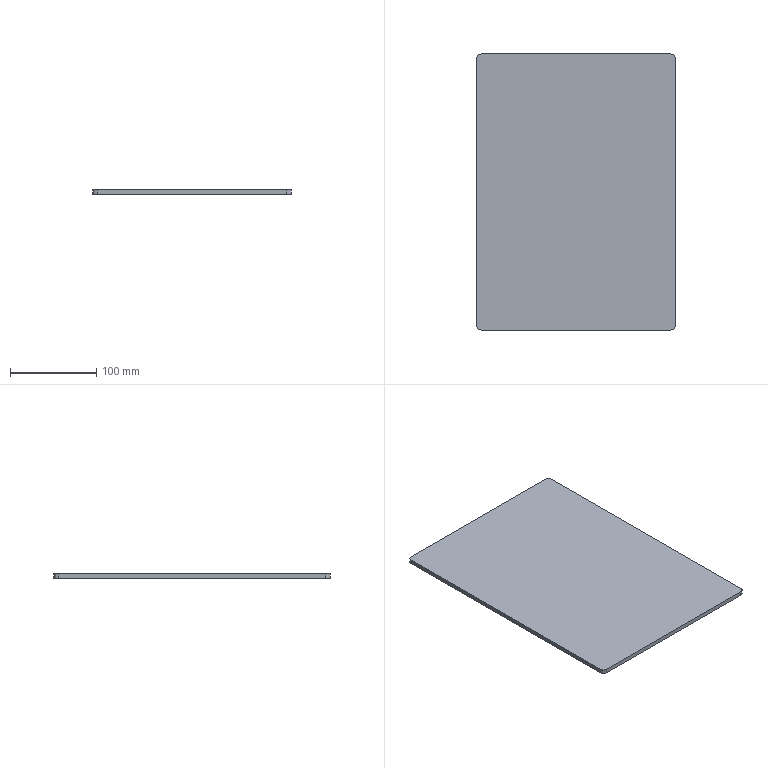Part | STEP file | 001-002-Face Plate-5 | 1 solid | 10 faces | box 230 x 320 x 5 mm | volume 367893 mm3 | plane 6 | cylinder 4 | commonest cylinder face diameters 10 x4
STEP:
#1=CARTESIAN_POINT('',(0.,0.,0.));
#2=DIRECTION('',(0.,0.,1.));
#3=DIRECTION('',(1.,0.,0.));
#4=AXIS2_PLACEMENT_3D('',#1,#2,#3);
#5=CARTESIAN_POINT('',(115.,-155.,0.));
#6=VERTEX_POINT('',#5);
#7=CARTESIAN_POINT('',(115.,155.,0.));
#8=VERTEX_POINT('',#7);
#9=CARTESIAN_POINT('',(115.,-160.,0.));
#10=DIRECTION('',(0.,1.,0.));
#11=VECTOR('',#10,1.);
#12=LINE('',#9,#11);
#13=CARTESIAN_POINT('',(115.,-160.,5.));
#14=DIRECTION('',(-1.,0.,0.));
#15=DIRECTION('',(0.,0.,1.));
#16=AXIS2_PLACEMENT_3D('',#13,#14,#15);
#17=PLANE('',#16);
#18=CARTESIAN_POINT('',(-5.,0.));
#19=DIRECTION('',(0.,1.));
#20=VECTOR('',#19,1.);
#21=LINE('',#18,#20);
#22=(GEOMETRIC_REPRESENTATION_CONTEXT(2)PARAMETRIC_REPRESENTATION_CONTEXT()REPRESENTATION_CONTEXT('',''));
#23=DEFINITIONAL_REPRESENTATION('',(#21),#22);
#24=PCURVE('',#17,#23);
#25=CARTESIAN_POINT('',(0.,0.,0.));
#26=DIRECTION('',(0.,0.,-1.));
#27=DIRECTION('',(-1.,0.,0.));
#28=AXIS2_PLACEMENT_3D('',#25,#26,#27);
#29=PLANE('',#28);
#30=CARTESIAN_POINT('',(-115.,-160.));
#31=DIRECTION('',(0.,1.));
#32=VECTOR('',#31,1.);
#33=LINE('',#30,#32);
#34=(GEOMETRIC_REPRESENTATION_CONTEXT(2)PARAMETRIC_REPRESENTATION_CONTEXT()REPRESENTATION_CONTEXT('',''));
#35=DEFINITIONAL_REPRESENTATION('',(#33),#34);
#36=PCURVE('',#29,#35);
#37=SURFACE_CURVE('',#12,(#24,#36),.PCURVE_S1.);
#38=EDGE_CURVE('',#6,#8,#37,.T.);
#39=ORIENTED_EDGE('',*,*,#38,.T.);
#40=CARTESIAN_POINT('',(115.,155.,5.));
#41=VERTEX_POINT('',#40);
#42=CARTESIAN_POINT('',(115.,155.,5.));
#43=DIRECTION('',(0.,0.,1.));
#44=VECTOR('',#43,1.);
#45=LINE('',#42,#44);
#46=CARTESIAN_POINT('',(0.,315.));
#47=DIRECTION('',(1.,0.));
#48=VECTOR('',#47,1.);
#49=LINE('',#46,#48);
#50=(GEOMETRIC_REPRESENTATION_CONTEXT(2)PARAMETRIC_REPRESENTATION_CONTEXT()REPRESENTATION_CONTEXT('',''));
#51=DEFINITIONAL_REPRESENTATION('',(#49),#50);
#52=PCURVE('',#17,#51);
#53=CARTESIAN_POINT('',(110.,155.,5.));
#54=DIRECTION('',(0.,0.,-1.));
#55=DIRECTION('',(-1.,0.,0.));
#56=AXIS2_PLACEMENT_3D('',#53,#54,#55);
#57=CYLINDRICAL_SURFACE('',#56,5.);
#58=CARTESIAN_POINT('',(3.142,0.));
#59=DIRECTION('',(0.,-1.));
#60=VECTOR('',#59,1.);
#61=LINE('',#58,#60);
#62=(GEOMETRIC_REPRESENTATION_CONTEXT(2)PARAMETRIC_REPRESENTATION_CONTEXT()REPRESENTATION_CONTEXT('',''));
#63=DEFINITIONAL_REPRESENTATION('',(#61),#62);
#64=PCURVE('',#57,#63);
#65=SURFACE_CURVE('',#45,(#52,#64),.PCURVE_S1.);
#66=EDGE_CURVE('',#8,#41,#65,.T.);
#67=ORIENTED_EDGE('',*,*,#66,.T.);
#68=CARTESIAN_POINT('',(115.,-155.,5.));
#69=VERTEX_POINT('',#68);
#70=CARTESIAN_POINT('',(115.,-160.,5.));
#71=DIRECTION('',(0.,1.,0.));
#72=VECTOR('',#71,1.);
#73=LINE('',#70,#72);
#74=CARTESIAN_POINT('',(0.,0.));
#75=DIRECTION('',(0.,1.));
#76=VECTOR('',#75,1.);
#77=LINE('',#74,#76);
#78=(GEOMETRIC_REPRESENTATION_CONTEXT(2)PARAMETRIC_REPRESENTATION_CONTEXT()REPRESENTATION_CONTEXT('',''));
#79=DEFINITIONAL_REPRESENTATION('',(#77),#78);
#80=PCURVE('',#17,#79);
#81=CARTESIAN_POINT('',(0.,0.,5.));
#82=DIRECTION('',(0.,0.,-1.));
#83=DIRECTION('',(-1.,0.,0.));
#84=AXIS2_PLACEMENT_3D('',#81,#82,#83);
#85=PLANE('',#84);
#86=CARTESIAN_POINT('',(-115.,-160.));
#87=DIRECTION('',(0.,1.));
#88=VECTOR('',#87,1.);
#89=LINE('',#86,#88);
#90=(GEOMETRIC_REPRESENTATION_CONTEXT(2)PARAMETRIC_REPRESENTATION_CONTEXT()REPRESENTATION_CONTEXT('',''));
#91=DEFINITIONAL_REPRESENTATION('',(#89),#90);
#92=PCURVE('',#85,#91);
#93=SURFACE_CURVE('',#73,(#80,#92),.PCURVE_S1.);
#94=EDGE_CURVE('',#69,#41,#93,.T.);
#95=ORIENTED_EDGE('',*,*,#94,.F.);
#96=CARTESIAN_POINT('',(115.,-155.,5.));
#97=DIRECTION('',(0.,0.,-1.));
#98=VECTOR('',#97,1.);
#99=LINE('',#96,#98);
#100=CARTESIAN_POINT('',(0.,5.));
#101=DIRECTION('',(-1.,0.));
#102=VECTOR('',#101,1.);
#103=LINE('',#100,#102);
#104=(GEOMETRIC_REPRESENTATION_CONTEXT(2)PARAMETRIC_REPRESENTATION_CONTEXT()REPRESENTATION_CONTEXT('',''));
#105=DEFINITIONAL_REPRESENTATION('',(#103),#104);
#106=PCURVE('',#17,#105);
#107=CARTESIAN_POINT('',(110.,-155.,5.));
#108=DIRECTION('',(0.,0.,-1.));
#109=DIRECTION('',(-1.,0.,0.));
#110=AXIS2_PLACEMENT_3D('',#107,#108,#109);
#111=CYLINDRICAL_SURFACE('',#110,5.);
#112=CARTESIAN_POINT('',(3.142,0.));
#113=DIRECTION('',(0.,1.));
#114=VECTOR('',#113,1.);
#115=LINE('',#112,#114);
#116=(GEOMETRIC_REPRESENTATION_CONTEXT(2)PARAMETRIC_REPRESENTATION_CONTEXT()REPRESENTATION_CONTEXT('',''));
#117=DEFINITIONAL_REPRESENTATION('',(#115),#116);
#118=PCURVE('',#111,#117);
#119=SURFACE_CURVE('',#99,(#106,#118),.PCURVE_S1.);
#120=EDGE_CURVE('',#69,#6,#119,.T.);
#121=ORIENTED_EDGE('',*,*,#120,.T.);
#122=EDGE_LOOP('',(#39,#67,#95,#121));
#123=FACE_BOUND('',#122,.T.);
#124=ADVANCED_FACE('',(#123),#17,.F.);
#125=CARTESIAN_POINT('',(110.,160.,0.));
#126=VERTEX_POINT('',#125);
#127=CARTESIAN_POINT('',(-110.,160.,0.));
#128=VERTEX_POINT('',#127);
#129=CARTESIAN_POINT('',(-115.,160.,0.));
#130=DIRECTION('',(-1.,0.,0.));
#131=VECTOR('',#130,1.);
#132=LINE('',#129,#131);
#133=CARTESIAN_POINT('',(-115.,160.,5.));
#134=DIRECTION('',(0.,-1.,0.));
#135=DIRECTION('',(0.,0.,-1.));
#136=AXIS2_PLACEMENT_3D('',#133,#134,#135);
#137=PLANE('',#136);
#138=CARTESIAN_POINT('',(5.,0.));
#139=DIRECTION('',(0.,-1.));
#140=VECTOR('',#139,1.);
#141=LINE('',#138,#140);
#142=(GEOMETRIC_REPRESENTATION_CONTEXT(2)PARAMETRIC_REPRESENTATION_CONTEXT()REPRESENTATION_CONTEXT('',''));
#143=DEFINITIONAL_REPRESENTATION('',(#141),#142);
#144=PCURVE('',#137,#143);
#145=CARTESIAN_POINT('',(115.,160.));
#146=DIRECTION('',(1.,0.));
#147=VECTOR('',#146,1.);
#148=LINE('',#145,#147);
#149=(GEOMETRIC_REPRESENTATION_CONTEXT(2)PARAMETRIC_REPRESENTATION_CONTEXT()REPRESENTATION_CONTEXT('',''));
#150=DEFINITIONAL_REPRESENTATION('',(#148),#149);
#151=PCURVE('',#29,#150);
#152=SURFACE_CURVE('',#132,(#144,#151),.PCURVE_S1.);
#153=EDGE_CURVE('',#126,#128,#152,.T.);
#154=ORIENTED_EDGE('',*,*,#153,.T.);
#155=CARTESIAN_POINT('',(-110.,160.,5.));
#156=VERTEX_POINT('',#155);
#157=CARTESIAN_POINT('',(-110.,160.,5.));
#158=DIRECTION('',(0.,0.,1.));
#159=VECTOR('',#158,1.);
#160=LINE('',#157,#159);
#161=CARTESIAN_POINT('',(0.,5.));
#162=DIRECTION('',(-1.,0.));
#163=VECTOR('',#162,1.);
#164=LINE('',#161,#163);
#165=(GEOMETRIC_REPRESENTATION_CONTEXT(2)PARAMETRIC_REPRESENTATION_CONTEXT()REPRESENTATION_CONTEXT('',''));
#166=DEFINITIONAL_REPRESENTATION('',(#164),#165);
#167=PCURVE('',#137,#166);
#168=CARTESIAN_POINT('',(-110.,155.,5.));
#169=DIRECTION('',(0.,0.,-1.));
#170=DIRECTION('',(-1.,0.,0.));
#171=AXIS2_PLACEMENT_3D('',#168,#169,#170);
#172=CYLINDRICAL_SURFACE('',#171,5.);
#173=CARTESIAN_POINT('',(1.571,0.));
#174=DIRECTION('',(0.,-1.));
#175=VECTOR('',#174,1.);
#176=LINE('',#173,#175);
#177=(GEOMETRIC_REPRESENTATION_CONTEXT(2)PARAMETRIC_REPRESENTATION_CONTEXT()REPRESENTATION_CONTEXT('',''));
#178=DEFINITIONAL_REPRESENTATION('',(#176),#177);
#179=PCURVE('',#172,#178);
#180=SURFACE_CURVE('',#160,(#167,#179),.PCURVE_S1.);
#181=EDGE_CURVE('',#128,#156,#180,.T.);
#182=ORIENTED_EDGE('',*,*,#181,.T.);
#183=CARTESIAN_POINT('',(110.,160.,5.));
#184=VERTEX_POINT('',#183);
#185=CARTESIAN_POINT('',(-115.,160.,5.));
#186=DIRECTION('',(-1.,0.,0.));
#187=VECTOR('',#186,1.);
#188=LINE('',#185,#187);
#189=CARTESIAN_POINT('',(0.,0.));
#190=DIRECTION('',(0.,-1.));
#191=VECTOR('',#190,1.);
#192=LINE('',#189,#191);
#193=(GEOMETRIC_REPRESENTATION_CONTEXT(2)PARAMETRIC_REPRESENTATION_CONTEXT()REPRESENTATION_CONTEXT('',''));
#194=DEFINITIONAL_REPRESENTATION('',(#192),#193);
#195=PCURVE('',#137,#194);
#196=CARTESIAN_POINT('',(115.,160.));
#197=DIRECTION('',(1.,0.));
#198=VECTOR('',#197,1.);
#199=LINE('',#196,#198);
#200=(GEOMETRIC_REPRESENTATION_CONTEXT(2)PARAMETRIC_REPRESENTATION_CONTEXT()REPRESENTATION_CONTEXT('',''));
#201=DEFINITIONAL_REPRESENTATION('',(#199),#200);
#202=PCURVE('',#85,#201);
#203=SURFACE_CURVE('',#188,(#195,#202),.PCURVE_S1.);
#204=EDGE_CURVE('',#184,#156,#203,.T.);
#205=ORIENTED_EDGE('',*,*,#204,.F.);
#206=CARTESIAN_POINT('',(110.,160.,5.));
#207=DIRECTION('',(0.,0.,-1.));
#208=VECTOR('',#207,1.);
#209=LINE('',#206,#208);
#210=CARTESIAN_POINT('',(0.,225.));
#211=DIRECTION('',(1.,0.));
#212=VECTOR('',#211,1.);
#213=LINE('',#210,#212);
#214=(GEOMETRIC_REPRESENTATION_CONTEXT(2)PARAMETRIC_REPRESENTATION_CONTEXT()REPRESENTATION_CONTEXT('',''));
#215=DEFINITIONAL_REPRESENTATION('',(#213),#214);
#216=PCURVE('',#137,#215);
#217=CARTESIAN_POINT('',(1.571,0.));
#218=DIRECTION('',(0.,1.));
#219=VECTOR('',#218,1.);
#220=LINE('',#217,#219);
#221=(GEOMETRIC_REPRESENTATION_CONTEXT(2)PARAMETRIC_REPRESENTATION_CONTEXT()REPRESENTATION_CONTEXT('',''));
#222=DEFINITIONAL_REPRESENTATION('',(#220),#221);
#223=PCURVE('',#57,#222);
#224=SURFACE_CURVE('',#209,(#216,#223),.PCURVE_S1.);
#225=EDGE_CURVE('',#184,#126,#224,.T.);
#226=ORIENTED_EDGE('',*,*,#225,.T.);
#227=EDGE_LOOP('',(#154,#182,#205,#226));
#228=FACE_BOUND('',#227,.T.);
#229=ADVANCED_FACE('',(#228),#137,.F.);
#230=CARTESIAN_POINT('',(-115.,155.,0.));
#231=VERTEX_POINT('',#230);
#232=CARTESIAN_POINT('',(-115.,-155.,0.));
#233=VERTEX_POINT('',#232);
#234=CARTESIAN_POINT('',(-115.,-160.,0.));
#235=DIRECTION('',(0.,-1.,0.));
#236=VECTOR('',#235,1.);
#237=LINE('',#234,#236);
#238=CARTESIAN_POINT('',(-115.,-160.,5.));
#239=DIRECTION('',(1.,0.,0.));
#240=DIRECTION('',(0.,0.,-1.));
#241=AXIS2_PLACEMENT_3D('',#238,#239,#240);
#242=PLANE('',#241);
#243=CARTESIAN_POINT('',(5.,0.));
#244=DIRECTION('',(0.,-1.));
#245=VECTOR('',#244,1.);
#246=LINE('',#243,#245);
#247=(GEOMETRIC_REPRESENTATION_CONTEXT(2)PARAMETRIC_REPRESENTATION_CONTEXT()REPRESENTATION_CONTEXT('',''));
#248=DEFINITIONAL_REPRESENTATION('',(#246),#247);
#249=PCURVE('',#242,#248);
#250=CARTESIAN_POINT('',(115.,-160.));
#251=DIRECTION('',(0.,-1.));
#252=VECTOR('',#251,1.);
#253=LINE('',#250,#252);
#254=(GEOMETRIC_REPRESENTATION_CONTEXT(2)PARAMETRIC_REPRESENTATION_CONTEXT()REPRESENTATION_CONTEXT('',''));
#255=DEFINITIONAL_REPRESENTATION('',(#253),#254);
#256=PCURVE('',#29,#255);
#257=SURFACE_CURVE('',#237,(#249,#256),.PCURVE_S1.);
#258=EDGE_CURVE('',#231,#233,#257,.T.);
#259=ORIENTED_EDGE('',*,*,#258,.T.);
#260=CARTESIAN_POINT('',(-115.,-155.,5.));
#261=VERTEX_POINT('',#260);
#262=CARTESIAN_POINT('',(-115.,-155.,5.));
#263=DIRECTION('',(0.,0.,1.));
#264=VECTOR('',#263,1.);
#265=LINE('',#262,#264);
#266=CARTESIAN_POINT('',(0.,5.));
#267=DIRECTION('',(-1.,0.));
#268=VECTOR('',#267,1.);
#269=LINE('',#266,#268);
#270=(GEOMETRIC_REPRESENTATION_CONTEXT(2)PARAMETRIC_REPRESENTATION_CONTEXT()REPRESENTATION_CONTEXT('',''));
#271=DEFINITIONAL_REPRESENTATION('',(#269),#270);
#272=PCURVE('',#242,#271);
#273=CARTESIAN_POINT('',(-110.,-155.,5.));
#274=DIRECTION('',(0.,0.,-1.));
#275=DIRECTION('',(-1.,0.,0.));
#276=AXIS2_PLACEMENT_3D('',#273,#274,#275);
#277=CYLINDRICAL_SURFACE('',#276,5.);
#278=CARTESIAN_POINT('',(6.283,0.));
#279=DIRECTION('',(0.,-1.));
#280=VECTOR('',#279,1.);
#281=LINE('',#278,#280);
#282=(GEOMETRIC_REPRESENTATION_CONTEXT(2)PARAMETRIC_REPRESENTATION_CONTEXT()REPRESENTATION_CONTEXT('',''));
#283=DEFINITIONAL_REPRESENTATION('',(#281),#282);
#284=PCURVE('',#277,#283);
#285=SURFACE_CURVE('',#265,(#272,#284),.PCURVE_S1.);
#286=EDGE_CURVE('',#233,#261,#285,.T.);
#287=ORIENTED_EDGE('',*,*,#286,.T.);
#288=CARTESIAN_POINT('',(-115.,155.,5.));
#289=VERTEX_POINT('',#288);
#290=CARTESIAN_POINT('',(-115.,-160.,5.));
#291=DIRECTION('',(0.,-1.,0.));
#292=VECTOR('',#291,1.);
#293=LINE('',#290,#292);
#294=CARTESIAN_POINT('',(0.,0.));
#295=DIRECTION('',(0.,-1.));
#296=VECTOR('',#295,1.);
#297=LINE('',#294,#296);
#298=(GEOMETRIC_REPRESENTATION_CONTEXT(2)PARAMETRIC_REPRESENTATION_CONTEXT()REPRESENTATION_CONTEXT('',''));
#299=DEFINITIONAL_REPRESENTATION('',(#297),#298);
#300=PCURVE('',#242,#299);
#301=CARTESIAN_POINT('',(115.,-160.));
#302=DIRECTION('',(0.,-1.));
#303=VECTOR('',#302,1.);
#304=LINE('',#301,#303);
#305=(GEOMETRIC_REPRESENTATION_CONTEXT(2)PARAMETRIC_REPRESENTATION_CONTEXT()REPRESENTATION_CONTEXT('',''));
#306=DEFINITIONAL_REPRESENTATION('',(#304),#305);
#307=PCURVE('',#85,#306);
#308=SURFACE_CURVE('',#293,(#300,#307),.PCURVE_S1.);
#309=EDGE_CURVE('',#289,#261,#308,.T.);
#310=ORIENTED_EDGE('',*,*,#309,.F.);
#311=CARTESIAN_POINT('',(-115.,155.,5.));
#312=DIRECTION('',(0.,0.,-1.));
#313=VECTOR('',#312,1.);
#314=LINE('',#311,#313);
#315=CARTESIAN_POINT('',(0.,315.));
#316=DIRECTION('',(1.,0.));
#317=VECTOR('',#316,1.);
#318=LINE('',#315,#317);
#319=(GEOMETRIC_REPRESENTATION_CONTEXT(2)PARAMETRIC_REPRESENTATION_CONTEXT()REPRESENTATION_CONTEXT('',''));
#320=DEFINITIONAL_REPRESENTATION('',(#318),#319);
#321=PCURVE('',#242,#320);
#322=CARTESIAN_POINT('',(0.,0.));
#323=DIRECTION('',(0.,1.));
#324=VECTOR('',#323,1.);
#325=LINE('',#322,#324);
#326=(GEOMETRIC_REPRESENTATION_CONTEXT(2)PARAMETRIC_REPRESENTATION_CONTEXT()REPRESENTATION_CONTEXT('',''));
#327=DEFINITIONAL_REPRESENTATION('',(#325),#326);
#328=PCURVE('',#172,#327);
#329=SURFACE_CURVE('',#314,(#321,#328),.PCURVE_S1.);
#330=EDGE_CURVE('',#289,#231,#329,.T.);
#331=ORIENTED_EDGE('',*,*,#330,.T.);
#332=EDGE_LOOP('',(#259,#287,#310,#331));
#333=FACE_BOUND('',#332,.T.);
#334=ADVANCED_FACE('',(#333),#242,.F.);
#335=CARTESIAN_POINT('',(-110.,-160.,5.));
#336=VERTEX_POINT('',#335);
#337=CARTESIAN_POINT('',(110.,-160.,5.));
#338=VERTEX_POINT('',#337);
#339=CARTESIAN_POINT('',(-115.,-160.,5.));
#340=DIRECTION('',(1.,0.,0.));
#341=VECTOR('',#340,1.);
#342=LINE('',#339,#341);
#343=CARTESIAN_POINT('',(-115.,-160.,5.));
#344=DIRECTION('',(0.,1.,0.));
#345=DIRECTION('',(0.,0.,1.));
#346=AXIS2_PLACEMENT_3D('',#343,#344,#345);
#347=PLANE('',#346);
#348=CARTESIAN_POINT('',(0.,0.));
#349=DIRECTION('',(0.,1.));
#350=VECTOR('',#349,1.);
#351=LINE('',#348,#350);
#352=(GEOMETRIC_REPRESENTATION_CONTEXT(2)PARAMETRIC_REPRESENTATION_CONTEXT()REPRESENTATION_CONTEXT('',''));
#353=DEFINITIONAL_REPRESENTATION('',(#351),#352);
#354=PCURVE('',#347,#353);
#355=CARTESIAN_POINT('',(115.,-160.));
#356=DIRECTION('',(-1.,0.));
#357=VECTOR('',#356,1.);
#358=LINE('',#355,#357);
#359=(GEOMETRIC_REPRESENTATION_CONTEXT(2)PARAMETRIC_REPRESENTATION_CONTEXT()REPRESENTATION_CONTEXT('',''));
#360=DEFINITIONAL_REPRESENTATION('',(#358),#359);
#361=PCURVE('',#85,#360);
#362=SURFACE_CURVE('',#342,(#354,#361),.PCURVE_S1.);
#363=EDGE_CURVE('',#336,#338,#362,.T.);
#364=ORIENTED_EDGE('',*,*,#363,.F.);
#365=CARTESIAN_POINT('',(-110.,-160.,0.));
#366=VERTEX_POINT('',#365);
#367=CARTESIAN_POINT('',(-110.,-160.,5.));
#368=DIRECTION('',(0.,0.,-1.));
#369=VECTOR('',#368,1.);
#370=LINE('',#367,#369);
#371=CARTESIAN_POINT('',(0.,5.));
#372=DIRECTION('',(-1.,0.));
#373=VECTOR('',#372,1.);
#374=LINE('',#371,#373);
#375=(GEOMETRIC_REPRESENTATION_CONTEXT(2)PARAMETRIC_REPRESENTATION_CONTEXT()REPRESENTATION_CONTEXT('',''));
#376=DEFINITIONAL_REPRESENTATION('',(#374),#375);
#377=PCURVE('',#347,#376);
#378=CARTESIAN_POINT('',(4.712,0.));
#379=DIRECTION('',(0.,1.));
#380=VECTOR('',#379,1.);
#381=LINE('',#378,#380);
#382=(GEOMETRIC_REPRESENTATION_CONTEXT(2)PARAMETRIC_REPRESENTATION_CONTEXT()REPRESENTATION_CONTEXT('',''));
#383=DEFINITIONAL_REPRESENTATION('',(#381),#382);
#384=PCURVE('',#277,#383);
#385=SURFACE_CURVE('',#370,(#377,#384),.PCURVE_S1.);
#386=EDGE_CURVE('',#336,#366,#385,.T.);
#387=ORIENTED_EDGE('',*,*,#386,.T.);
#388=CARTESIAN_POINT('',(110.,-160.,0.));
#389=VERTEX_POINT('',#388);
#390=CARTESIAN_POINT('',(-115.,-160.,0.));
#391=DIRECTION('',(1.,0.,0.));
#392=VECTOR('',#391,1.);
#393=LINE('',#390,#392);
#394=CARTESIAN_POINT('',(-5.,0.));
#395=DIRECTION('',(0.,1.));
#396=VECTOR('',#395,1.);
#397=LINE('',#394,#396);
#398=(GEOMETRIC_REPRESENTATION_CONTEXT(2)PARAMETRIC_REPRESENTATION_CONTEXT()REPRESENTATION_CONTEXT('',''));
#399=DEFINITIONAL_REPRESENTATION('',(#397),#398);
#400=PCURVE('',#347,#399);
#401=CARTESIAN_POINT('',(115.,-160.));
#402=DIRECTION('',(-1.,0.));
#403=VECTOR('',#402,1.);
#404=LINE('',#401,#403);
#405=(GEOMETRIC_REPRESENTATION_CONTEXT(2)PARAMETRIC_REPRESENTATION_CONTEXT()REPRESENTATION_CONTEXT('',''));
#406=DEFINITIONAL_REPRESENTATION('',(#404),#405);
#407=PCURVE('',#29,#406);
#408=SURFACE_CURVE('',#393,(#400,#407),.PCURVE_S1.);
#409=EDGE_CURVE('',#366,#389,#408,.T.);
#410=ORIENTED_EDGE('',*,*,#409,.T.);
#411=CARTESIAN_POINT('',(110.,-160.,5.));
#412=DIRECTION('',(0.,0.,1.));
#413=VECTOR('',#412,1.);
#414=LINE('',#411,#413);
#415=CARTESIAN_POINT('',(0.,225.));
#416=DIRECTION('',(1.,0.));
#417=VECTOR('',#416,1.);
#418=LINE('',#415,#417);
#419=(GEOMETRIC_REPRESENTATION_CONTEXT(2)PARAMETRIC_REPRESENTATION_CONTEXT()REPRESENTATION_CONTEXT('',''));
#420=DEFINITIONAL_REPRESENTATION('',(#418),#419);
#421=PCURVE('',#347,#420);
#422=CARTESIAN_POINT('',(4.712,0.));
#423=DIRECTION('',(0.,-1.));
#424=VECTOR('',#423,1.);
#425=LINE('',#422,#424);
#426=(GEOMETRIC_REPRESENTATION_CONTEXT(2)PARAMETRIC_REPRESENTATION_CONTEXT()REPRESENTATION_CONTEXT('',''));
#427=DEFINITIONAL_REPRESENTATION('',(#425),#426);
#428=PCURVE('',#111,#427);
#429=SURFACE_CURVE('',#414,(#421,#428),.PCURVE_S1.);
#430=EDGE_CURVE('',#389,#338,#429,.T.);
#431=ORIENTED_EDGE('',*,*,#430,.T.);
#432=EDGE_LOOP('',(#364,#387,#410,#431));
#433=FACE_BOUND('',#432,.T.);
#434=ADVANCED_FACE('',(#433),#347,.F.);
#435=ORIENTED_EDGE('',*,*,#309,.T.);
#436=CARTESIAN_POINT('',(-110.,-155.,5.));
#437=DIRECTION('',(0.,0.,1.));
#438=DIRECTION('',(-1.,0.,0.));
#439=AXIS2_PLACEMENT_3D('',#436,#437,#438);
#440=CIRCLE('',#439,5.);
#441=CARTESIAN_POINT('',(115.,-155.));
#442=CARTESIAN_POINT('',(115.,-163.66));
#443=CARTESIAN_POINT('',(107.5,-159.33));
#444=CARTESIAN_POINT('',(100.,-155.));
#445=CARTESIAN_POINT('',(107.5,-150.67));
#446=CARTESIAN_POINT('',(115.,-146.34));
#447=CARTESIAN_POINT('',(115.,-155.));
#448=(BOUNDED_CURVE()B_SPLINE_CURVE(2,(#441,#442,#443,#444,#445,#446,#447),.UNSPECIFIED.,.T.,.F.)B_SPLINE_CURVE_WITH_KNOTS((1,2,2,2,2,1),(-2.094,0.,2.094,4.189,6.283,8.378),.UNSPECIFIED.)CURVE()GEOMETRIC_REPRESENTATION_ITEM()RATIONAL_B_SPLINE_CURVE((1.,0.5,1.,0.5,1.,0.5,1.))REPRESENTATION_ITEM(''));
#449=(GEOMETRIC_REPRESENTATION_CONTEXT(2)PARAMETRIC_REPRESENTATION_CONTEXT()REPRESENTATION_CONTEXT('',''));
#450=DEFINITIONAL_REPRESENTATION('',(#448),#449);
#451=PCURVE('',#85,#450);
#452=CARTESIAN_POINT('',(6.283,0.));
#453=DIRECTION('',(-1.,0.));
#454=VECTOR('',#453,1.);
#455=LINE('',#452,#454);
#456=(GEOMETRIC_REPRESENTATION_CONTEXT(2)PARAMETRIC_REPRESENTATION_CONTEXT()REPRESENTATION_CONTEXT('',''));
#457=DEFINITIONAL_REPRESENTATION('',(#455),#456);
#458=PCURVE('',#277,#457);
#459=SURFACE_CURVE('',#440,(#451,#458),.PCURVE_S1.);
#460=EDGE_CURVE('',#261,#336,#459,.T.);
#461=ORIENTED_EDGE('',*,*,#460,.T.);
#462=ORIENTED_EDGE('',*,*,#363,.T.);
#463=CARTESIAN_POINT('',(110.,-155.,5.));
#464=DIRECTION('',(0.,0.,1.));
#465=DIRECTION('',(-1.,0.,0.));
#466=AXIS2_PLACEMENT_3D('',#463,#464,#465);
#467=CIRCLE('',#466,5.);
#468=CARTESIAN_POINT('',(-105.,-155.));
#469=CARTESIAN_POINT('',(-105.,-163.66));
#470=CARTESIAN_POINT('',(-112.5,-159.33));
#471=CARTESIAN_POINT('',(-120.,-155.));
#472=CARTESIAN_POINT('',(-112.5,-150.67));
#473=CARTESIAN_POINT('',(-105.,-146.34));
#474=CARTESIAN_POINT('',(-105.,-155.));
#475=(BOUNDED_CURVE()B_SPLINE_CURVE(2,(#468,#469,#470,#471,#472,#473,#474),.UNSPECIFIED.,.T.,.F.)B_SPLINE_CURVE_WITH_KNOTS((1,2,2,2,2,1),(-2.094,0.,2.094,4.189,6.283,8.378),.UNSPECIFIED.)CURVE()GEOMETRIC_REPRESENTATION_ITEM()RATIONAL_B_SPLINE_CURVE((1.,0.5,1.,0.5,1.,0.5,1.))REPRESENTATION_ITEM(''));
#476=(GEOMETRIC_REPRESENTATION_CONTEXT(2)PARAMETRIC_REPRESENTATION_CONTEXT()REPRESENTATION_CONTEXT('',''));
#477=DEFINITIONAL_REPRESENTATION('',(#475),#476);
#478=PCURVE('',#85,#477);
#479=CARTESIAN_POINT('',(6.283,0.));
#480=DIRECTION('',(-1.,0.));
#481=VECTOR('',#480,1.);
#482=LINE('',#479,#481);
#483=(GEOMETRIC_REPRESENTATION_CONTEXT(2)PARAMETRIC_REPRESENTATION_CONTEXT()REPRESENTATION_CONTEXT('',''));
#484=DEFINITIONAL_REPRESENTATION('',(#482),#483);
#485=PCURVE('',#111,#484);
#486=SURFACE_CURVE('',#467,(#478,#485),.PCURVE_S1.);
#487=EDGE_CURVE('',#338,#69,#486,.T.);
#488=ORIENTED_EDGE('',*,*,#487,.T.);
#489=ORIENTED_EDGE('',*,*,#94,.T.);
#490=CARTESIAN_POINT('',(110.,155.,5.));
#491=DIRECTION('',(0.,0.,1.));
#492=DIRECTION('',(-1.,0.,0.));
#493=AXIS2_PLACEMENT_3D('',#490,#491,#492);
#494=CIRCLE('',#493,5.);
#495=CARTESIAN_POINT('',(-105.,155.));
#496=CARTESIAN_POINT('',(-105.,146.34));
#497=CARTESIAN_POINT('',(-112.5,150.67));
#498=CARTESIAN_POINT('',(-120.,155.));
#499=CARTESIAN_POINT('',(-112.5,159.33));
#500=CARTESIAN_POINT('',(-105.,163.66));
#501=CARTESIAN_POINT('',(-105.,155.));
#502=(BOUNDED_CURVE()B_SPLINE_CURVE(2,(#495,#496,#497,#498,#499,#500,#501),.UNSPECIFIED.,.T.,.F.)B_SPLINE_CURVE_WITH_KNOTS((1,2,2,2,2,1),(-2.094,0.,2.094,4.189,6.283,8.378),.UNSPECIFIED.)CURVE()GEOMETRIC_REPRESENTATION_ITEM()RATIONAL_B_SPLINE_CURVE((1.,0.5,1.,0.5,1.,0.5,1.))REPRESENTATION_ITEM(''));
#503=(GEOMETRIC_REPRESENTATION_CONTEXT(2)PARAMETRIC_REPRESENTATION_CONTEXT()REPRESENTATION_CONTEXT('',''));
#504=DEFINITIONAL_REPRESENTATION('',(#502),#503);
#505=PCURVE('',#85,#504);
#506=CARTESIAN_POINT('',(6.283,0.));
#507=DIRECTION('',(-1.,0.));
#508=VECTOR('',#507,1.);
#509=LINE('',#506,#508);
#510=(GEOMETRIC_REPRESENTATION_CONTEXT(2)PARAMETRIC_REPRESENTATION_CONTEXT()REPRESENTATION_CONTEXT('',''));
#511=DEFINITIONAL_REPRESENTATION('',(#509),#510);
#512=PCURVE('',#57,#511);
#513=SURFACE_CURVE('',#494,(#505,#512),.PCURVE_S1.);
#514=EDGE_CURVE('',#41,#184,#513,.T.);
#515=ORIENTED_EDGE('',*,*,#514,.T.);
#516=ORIENTED_EDGE('',*,*,#204,.T.);
#517=CARTESIAN_POINT('',(-110.,155.,5.));
#518=DIRECTION('',(0.,0.,1.));
#519=DIRECTION('',(-1.,0.,0.));
#520=AXIS2_PLACEMENT_3D('',#517,#518,#519);
#521=CIRCLE('',#520,5.);
#522=CARTESIAN_POINT('',(115.,155.));
#523=CARTESIAN_POINT('',(115.,146.34));
#524=CARTESIAN_POINT('',(107.5,150.67));
#525=CARTESIAN_POINT('',(100.,155.));
#526=CARTESIAN_POINT('',(107.5,159.33));
#527=CARTESIAN_POINT('',(115.,163.66));
#528=CARTESIAN_POINT('',(115.,155.));
#529=(BOUNDED_CURVE()B_SPLINE_CURVE(2,(#522,#523,#524,#525,#526,#527,#528),.UNSPECIFIED.,.T.,.F.)B_SPLINE_CURVE_WITH_KNOTS((1,2,2,2,2,1),(-2.094,0.,2.094,4.189,6.283,8.378),.UNSPECIFIED.)CURVE()GEOMETRIC_REPRESENTATION_ITEM()RATIONAL_B_SPLINE_CURVE((1.,0.5,1.,0.5,1.,0.5,1.))REPRESENTATION_ITEM(''));
#530=(GEOMETRIC_REPRESENTATION_CONTEXT(2)PARAMETRIC_REPRESENTATION_CONTEXT()REPRESENTATION_CONTEXT('',''));
#531=DEFINITIONAL_REPRESENTATION('',(#529),#530);
#532=PCURVE('',#85,#531);
#533=CARTESIAN_POINT('',(6.283,0.));
#534=DIRECTION('',(-1.,0.));
#535=VECTOR('',#534,1.);
#536=LINE('',#533,#535);
#537=(GEOMETRIC_REPRESENTATION_CONTEXT(2)PARAMETRIC_REPRESENTATION_CONTEXT()REPRESENTATION_CONTEXT('',''));
#538=DEFINITIONAL_REPRESENTATION('',(#536),#537);
#539=PCURVE('',#172,#538);
#540=SURFACE_CURVE('',#521,(#532,#539),.PCURVE_S1.);
#541=EDGE_CURVE('',#156,#289,#540,.T.);
#542=ORIENTED_EDGE('',*,*,#541,.T.);
#543=EDGE_LOOP('',(#435,#461,#462,#488,#489,#515,#516,#542));
#544=FACE_BOUND('',#543,.T.);
#545=ADVANCED_FACE('',(#544),#85,.F.);
#546=ORIENTED_EDGE('',*,*,#409,.F.);
#547=CARTESIAN_POINT('',(-110.,-155.,0.));
#548=DIRECTION('',(0.,0.,-1.));
#549=DIRECTION('',(-1.,0.,0.));
#550=AXIS2_PLACEMENT_3D('',#547,#548,#549);
#551=CIRCLE('',#550,5.);
#552=CARTESIAN_POINT('',(110.,-155.));
#553=DIRECTION('',(1.,0.));
#554=AXIS2_PLACEMENT_2D('',#552,#553);
#555=CIRCLE('',#554,5.);
#556=(GEOMETRIC_REPRESENTATION_CONTEXT(2)PARAMETRIC_REPRESENTATION_CONTEXT()REPRESENTATION_CONTEXT('',''));
#557=DEFINITIONAL_REPRESENTATION('',(#555),#556);
#558=PCURVE('',#29,#557);
#559=CARTESIAN_POINT('',(0.,5.));
#560=DIRECTION('',(1.,0.));
#561=VECTOR('',#560,1.);
#562=LINE('',#559,#561);
#563=(GEOMETRIC_REPRESENTATION_CONTEXT(2)PARAMETRIC_REPRESENTATION_CONTEXT()REPRESENTATION_CONTEXT('',''));
#564=DEFINITIONAL_REPRESENTATION('',(#562),#563);
#565=PCURVE('',#277,#564);
#566=SURFACE_CURVE('',#551,(#558,#565),.PCURVE_S1.);
#567=EDGE_CURVE('',#366,#233,#566,.T.);
#568=ORIENTED_EDGE('',*,*,#567,.T.);
#569=ORIENTED_EDGE('',*,*,#258,.F.);
#570=CARTESIAN_POINT('',(-110.,155.,0.));
#571=DIRECTION('',(0.,0.,-1.));
#572=DIRECTION('',(-1.,0.,0.));
#573=AXIS2_PLACEMENT_3D('',#570,#571,#572);
#574=CIRCLE('',#573,5.);
#575=CARTESIAN_POINT('',(110.,155.));
#576=DIRECTION('',(1.,0.));
#577=AXIS2_PLACEMENT_2D('',#575,#576);
#578=CIRCLE('',#577,5.);
#579=(GEOMETRIC_REPRESENTATION_CONTEXT(2)PARAMETRIC_REPRESENTATION_CONTEXT()REPRESENTATION_CONTEXT('',''));
#580=DEFINITIONAL_REPRESENTATION('',(#578),#579);
#581=PCURVE('',#29,#580);
#582=CARTESIAN_POINT('',(0.,5.));
#583=DIRECTION('',(1.,0.));
#584=VECTOR('',#583,1.);
#585=LINE('',#582,#584);
#586=(GEOMETRIC_REPRESENTATION_CONTEXT(2)PARAMETRIC_REPRESENTATION_CONTEXT()REPRESENTATION_CONTEXT('',''));
#587=DEFINITIONAL_REPRESENTATION('',(#585),#586);
#588=PCURVE('',#172,#587);
#589=SURFACE_CURVE('',#574,(#581,#588),.PCURVE_S1.);
#590=EDGE_CURVE('',#231,#128,#589,.T.);
#591=ORIENTED_EDGE('',*,*,#590,.T.);
#592=ORIENTED_EDGE('',*,*,#153,.F.);
#593=CARTESIAN_POINT('',(110.,155.,0.));
#594=DIRECTION('',(0.,0.,-1.));
#595=DIRECTION('',(-1.,0.,0.));
#596=AXIS2_PLACEMENT_3D('',#593,#594,#595);
#597=CIRCLE('',#596,5.);
#598=CARTESIAN_POINT('',(-110.,155.));
#599=DIRECTION('',(1.,0.));
#600=AXIS2_PLACEMENT_2D('',#598,#599);
#601=CIRCLE('',#600,5.);
#602=(GEOMETRIC_REPRESENTATION_CONTEXT(2)PARAMETRIC_REPRESENTATION_CONTEXT()REPRESENTATION_CONTEXT('',''));
#603=DEFINITIONAL_REPRESENTATION('',(#601),#602);
#604=PCURVE('',#29,#603);
#605=CARTESIAN_POINT('',(0.,5.));
#606=DIRECTION('',(1.,0.));
#607=VECTOR('',#606,1.);
#608=LINE('',#605,#607);
#609=(GEOMETRIC_REPRESENTATION_CONTEXT(2)PARAMETRIC_REPRESENTATION_CONTEXT()REPRESENTATION_CONTEXT('',''));
#610=DEFINITIONAL_REPRESENTATION('',(#608),#609);
#611=PCURVE('',#57,#610);
#612=SURFACE_CURVE('',#597,(#604,#611),.PCURVE_S1.);
#613=EDGE_CURVE('',#126,#8,#612,.T.);
#614=ORIENTED_EDGE('',*,*,#613,.T.);
#615=ORIENTED_EDGE('',*,*,#38,.F.);
#616=CARTESIAN_POINT('',(110.,-155.,0.));
#617=DIRECTION('',(0.,0.,-1.));
#618=DIRECTION('',(-1.,0.,0.));
#619=AXIS2_PLACEMENT_3D('',#616,#617,#618);
#620=CIRCLE('',#619,5.);
#621=CARTESIAN_POINT('',(-110.,-155.));
#622=DIRECTION('',(1.,0.));
#623=AXIS2_PLACEMENT_2D('',#621,#622);
#624=CIRCLE('',#623,5.);
#625=(GEOMETRIC_REPRESENTATION_CONTEXT(2)PARAMETRIC_REPRESENTATION_CONTEXT()REPRESENTATION_CONTEXT('',''));
#626=DEFINITIONAL_REPRESENTATION('',(#624),#625);
#627=PCURVE('',#29,#626);
#628=CARTESIAN_POINT('',(0.,5.));
#629=DIRECTION('',(1.,0.));
#630=VECTOR('',#629,1.);
#631=LINE('',#628,#630);
#632=(GEOMETRIC_REPRESENTATION_CONTEXT(2)PARAMETRIC_REPRESENTATION_CONTEXT()REPRESENTATION_CONTEXT('',''));
#633=DEFINITIONAL_REPRESENTATION('',(#631),#632);
#634=PCURVE('',#111,#633);
#635=SURFACE_CURVE('',#620,(#627,#634),.PCURVE_S1.);
#636=EDGE_CURVE('',#6,#389,#635,.T.);
#637=ORIENTED_EDGE('',*,*,#636,.T.);
#638=EDGE_LOOP('',(#546,#568,#569,#591,#592,#614,#615,#637));
#639=FACE_BOUND('',#638,.T.);
#640=ADVANCED_FACE('',(#639),#29,.T.);
#641=ORIENTED_EDGE('',*,*,#460,.F.);
#642=ORIENTED_EDGE('',*,*,#286,.F.);
#643=ORIENTED_EDGE('',*,*,#567,.F.);
#644=ORIENTED_EDGE('',*,*,#386,.F.);
#645=EDGE_LOOP('',(#641,#642,#643,#644));
#646=FACE_BOUND('',#645,.T.);
#647=ADVANCED_FACE('',(#646),#277,.T.);
#648=ORIENTED_EDGE('',*,*,#541,.F.);
#649=ORIENTED_EDGE('',*,*,#181,.F.);
#650=ORIENTED_EDGE('',*,*,#590,.F.);
#651=ORIENTED_EDGE('',*,*,#330,.F.);
#652=EDGE_LOOP('',(#648,#649,#650,#651));
#653=FACE_BOUND('',#652,.T.);
#654=ADVANCED_FACE('',(#653),#172,.T.);
#655=ORIENTED_EDGE('',*,*,#514,.F.);
#656=ORIENTED_EDGE('',*,*,#66,.F.);
#657=ORIENTED_EDGE('',*,*,#613,.F.);
#658=ORIENTED_EDGE('',*,*,#225,.F.);
#659=EDGE_LOOP('',(#655,#656,#657,#658));
#660=FACE_BOUND('',#659,.T.);
#661=ADVANCED_FACE('',(#660),#57,.T.);
#662=ORIENTED_EDGE('',*,*,#487,.F.);
#663=ORIENTED_EDGE('',*,*,#430,.F.);
#664=ORIENTED_EDGE('',*,*,#636,.F.);
#665=ORIENTED_EDGE('',*,*,#120,.F.);
#666=EDGE_LOOP('',(#662,#663,#664,#665));
#667=FACE_BOUND('',#666,.T.);
#668=ADVANCED_FACE('',(#667),#111,.T.);
#669=CLOSED_SHELL('',(#124,#229,#334,#434,#545,#640,#647,#654,#661,#668));
#670=MANIFOLD_SOLID_BREP('',#669);
#671=(LENGTH_UNIT()NAMED_UNIT(*)SI_UNIT(.MILLI.,.METRE.));
#672=UNCERTAINTY_MEASURE_WITH_UNIT(LENGTH_MEASURE(0.0000001),#671,'','');
#673=(NAMED_UNIT(*)PLANE_ANGLE_UNIT()SI_UNIT($,.RADIAN.));
#674=(NAMED_UNIT(*)SI_UNIT($,.STERADIAN.)SOLID_ANGLE_UNIT());
#675=(GEOMETRIC_REPRESENTATION_CONTEXT(3)GLOBAL_UNCERTAINTY_ASSIGNED_CONTEXT((#672))GLOBAL_UNIT_ASSIGNED_CONTEXT((#671,#673,#674))REPRESENTATION_CONTEXT('',''));
#676=ADVANCED_BREP_SHAPE_REPRESENTATION('',(#4,#670),#675);